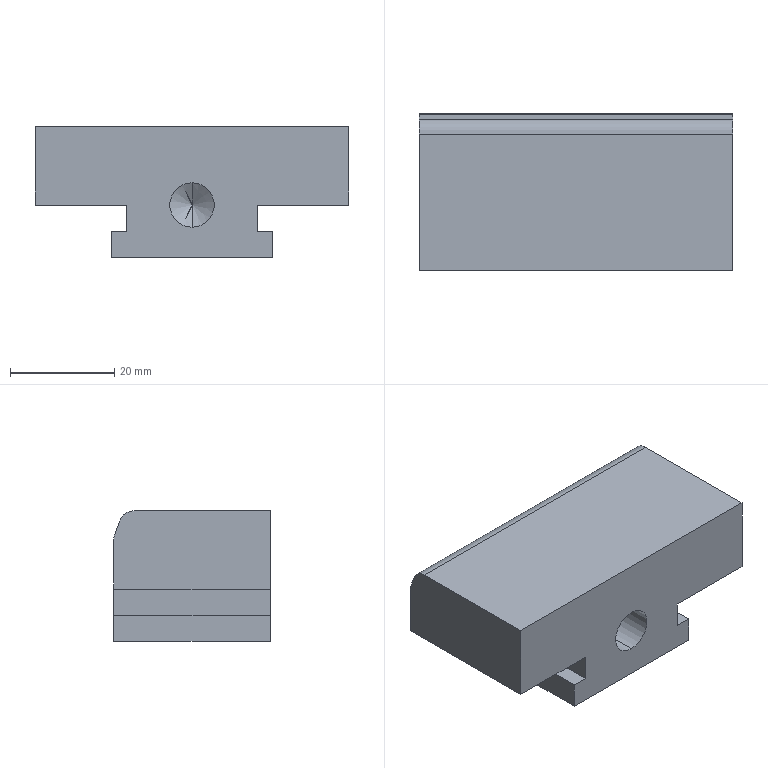Part | SolidWorks | features Chamfer 1, Cut 1, Extrusion 1, Fillet 1, HoleWzd 1, ICE 1 | 1 solid | 21 faces | box 60 x 30 x 25 mm | volume 33639 mm3 | plane 15 | cylinder 4 | cone 2 | commonest cylinder face diameters 6 x2 8.5 x2
STEP:
#1=CARTESIAN_POINT('',(-16.517,24.697,14.25));
#2=VERTEX_POINT('',#1);
#3=CARTESIAN_POINT('',(-16.517,24.697,5.75));
#4=VERTEX_POINT('',#3);
#5=CARTESIAN_POINT('',(-16.517,24.697,10.));
#6=DIRECTION('',(0.,-1.,0.));
#7=DIRECTION('',(0.,0.,-1.));
#8=AXIS2_PLACEMENT_3D('',#5,#6,#7);
#9=CIRCLE('',#8,4.25);
#10=EDGE_CURVE('',#2,#4,#9,.T.);
#11=ORIENTED_EDGE('',*,*,#10,.F.);
#12=CARTESIAN_POINT('',(-16.517,0.1974,14.25));
#13=VERTEX_POINT('',#12);
#14=CARTESIAN_POINT('',(-16.517,0.1974,14.25));
#15=DIRECTION('',(0.,-1.,0.));
#16=VECTOR('',#15,1000.);
#17=LINE('',#14,#16);
#18=EDGE_CURVE('',#2,#13,#17,.T.);
#19=ORIENTED_EDGE('',*,*,#18,.T.);
#20=CARTESIAN_POINT('',(-16.517,0.1974,5.75));
#21=VERTEX_POINT('',#20);
#22=CARTESIAN_POINT('',(-16.517,0.1974,10.));
#23=DIRECTION('',(0.,-1.,0.));
#24=DIRECTION('',(0.,0.,-1.));
#25=AXIS2_PLACEMENT_3D('',#22,#23,#24);
#26=CIRCLE('',#25,4.25);
#27=EDGE_CURVE('',#13,#21,#26,.T.);
#28=ORIENTED_EDGE('',*,*,#27,.T.);
#29=CARTESIAN_POINT('',(-16.517,0.1974,5.75));
#30=DIRECTION('',(0.,-1.,0.));
#31=VECTOR('',#30,1000.);
#32=LINE('',#29,#31);
#33=EDGE_CURVE('',#4,#21,#32,.T.);
#34=ORIENTED_EDGE('',*,*,#33,.F.);
#35=EDGE_LOOP('',(#11,#19,#28,#34));
#36=FACE_OUTER_BOUND('',#35,.T.);
#37=CARTESIAN_POINT('',(-16.517,0.1974,10.));
#38=DIRECTION('',(0.,-1.,0.));
#39=DIRECTION('',(0.,0.,-1.));
#40=AXIS2_PLACEMENT_3D('',#37,#38,#39);
#41=CYLINDRICAL_SURFACE('',#40,4.25);
#42=ADVANCED_FACE('',(#36),#41,.F.);
#43=CARTESIAN_POINT('',(-16.517,27.251,10.));
#44=VERTEX_POINT('',#43);
#45=CARTESIAN_POINT('',(-16.517,24.697,5.75));
#46=DIRECTION('',(0.,-0.515,-0.8572));
#47=VECTOR('',#46,1000.);
#48=LINE('',#45,#47);
#49=EDGE_CURVE('',#44,#4,#48,.T.);
#50=ORIENTED_EDGE('',*,*,#49,.F.);
#51=CARTESIAN_POINT('',(-16.517,24.697,14.25));
#52=DIRECTION('',(0.,-0.515,0.8572));
#53=VECTOR('',#52,1000.);
#54=LINE('',#51,#53);
#55=EDGE_CURVE('',#44,#2,#54,.T.);
#56=ORIENTED_EDGE('',*,*,#55,.T.);
#57=ORIENTED_EDGE('',*,*,#10,.T.);
#58=EDGE_LOOP('',(#50,#56,#57));
#59=FACE_OUTER_BOUND('',#58,.T.);
#60=CARTESIAN_POINT('',(-16.517,24.697,10.));
#61=DIRECTION('',(0.,-1.,0.));
#62=DIRECTION('',(0.,0.,-1.));
#63=AXIS2_PLACEMENT_3D('',#60,#61,#62);
#64=CONICAL_SURFACE('',#63,4.25,1.03);
#65=ADVANCED_FACE('',(#59),#64,.F.);
#66=CARTESIAN_POINT('',(-32.017,0.1974,5.));
#67=VERTEX_POINT('',#66);
#68=CARTESIAN_POINT('',(-32.017,0.1974,0.));
#69=VERTEX_POINT('',#68);
#70=CARTESIAN_POINT('',(-32.017,0.1974,25.));
#71=DIRECTION('',(0.,0.,-1.));
#72=VECTOR('',#71,1000.);
#73=LINE('',#70,#72);
#74=EDGE_CURVE('',#67,#69,#73,.T.);
#75=ORIENTED_EDGE('',*,*,#74,.F.);
#76=CARTESIAN_POINT('',(-32.017,30.197,5.));
#77=VERTEX_POINT('',#76);
#78=CARTESIAN_POINT('',(-32.017,30.197,5.));
#79=DIRECTION('',(0.,-1.,0.));
#80=VECTOR('',#79,1000.);
#81=LINE('',#78,#80);
#82=EDGE_CURVE('',#77,#67,#81,.T.);
#83=ORIENTED_EDGE('',*,*,#82,.F.);
#84=CARTESIAN_POINT('',(-32.017,30.197,0.));
#85=VERTEX_POINT('',#84);
#86=CARTESIAN_POINT('',(-32.017,30.197,25.));
#87=DIRECTION('',(0.,0.,-1.));
#88=VECTOR('',#87,1000.);
#89=LINE('',#86,#88);
#90=EDGE_CURVE('',#77,#85,#89,.T.);
#91=ORIENTED_EDGE('',*,*,#90,.T.);
#92=CARTESIAN_POINT('',(-32.017,30.197,0.));
#93=DIRECTION('',(0.,-1.,0.));
#94=VECTOR('',#93,1000.);
#95=LINE('',#92,#94);
#96=EDGE_CURVE('',#85,#69,#95,.T.);
#97=ORIENTED_EDGE('',*,*,#96,.T.);
#98=EDGE_LOOP('',(#75,#83,#91,#97));
#99=FACE_OUTER_BOUND('',#98,.T.);
#100=CARTESIAN_POINT('',(-32.017,30.197,25.));
#101=DIRECTION('',(1.,0.,0.));
#102=DIRECTION('',(0.,1.,0.));
#103=AXIS2_PLACEMENT_3D('',#100,#101,#102);
#104=PLANE('',#103);
#105=ADVANCED_FACE('',(#99),#104,.F.);
#106=CARTESIAN_POINT('',(-16.517,0.1974,10.));
#107=DIRECTION('',(0.,-1.,0.));
#108=DIRECTION('',(0.,0.,-1.));
#109=AXIS2_PLACEMENT_3D('',#106,#107,#108);
#110=CIRCLE('',#109,4.25);
#111=EDGE_CURVE('',#21,#13,#110,.T.);
#112=ORIENTED_EDGE('',*,*,#111,.F.);
#113=ORIENTED_EDGE('',*,*,#27,.F.);
#114=EDGE_LOOP('',(#112,#113));
#115=FACE_BOUND('',#114,.T.);
#116=CARTESIAN_POINT('',(-4.017,0.1974,5.));
#117=VERTEX_POINT('',#116);
#118=CARTESIAN_POINT('',(-1.017,0.1974,5.));
#119=VERTEX_POINT('',#118);
#120=CARTESIAN_POINT('',(-4.017,0.1974,5.));
#121=DIRECTION('',(1.,0.,0.));
#122=VECTOR('',#121,1000.);
#123=LINE('',#120,#122);
#124=EDGE_CURVE('',#117,#119,#123,.T.);
#125=ORIENTED_EDGE('',*,*,#124,.F.);
#126=CARTESIAN_POINT('',(-4.017,0.1974,10.));
#127=VERTEX_POINT('',#126);
#128=CARTESIAN_POINT('',(-4.017,0.1974,5.));
#129=DIRECTION('',(0.,0.,-1.));
#130=VECTOR('',#129,1000.);
#131=LINE('',#128,#130);
#132=EDGE_CURVE('',#127,#117,#131,.T.);
#133=ORIENTED_EDGE('',*,*,#132,.F.);
#134=CARTESIAN_POINT('',(13.483,0.1974,10.));
#135=VERTEX_POINT('',#134);
#136=CARTESIAN_POINT('',(-4.017,0.1974,10.));
#137=DIRECTION('',(-1.,0.,0.));
#138=VECTOR('',#137,1000.);
#139=LINE('',#136,#138);
#140=EDGE_CURVE('',#135,#127,#139,.T.);
#141=ORIENTED_EDGE('',*,*,#140,.F.);
#142=CARTESIAN_POINT('',(13.483,0.1974,25.));
#143=VERTEX_POINT('',#142);
#144=CARTESIAN_POINT('',(13.483,0.1974,25.));
#145=DIRECTION('',(0.,0.,-1.));
#146=VECTOR('',#145,1000.);
#147=LINE('',#144,#146);
#148=EDGE_CURVE('',#143,#135,#147,.T.);
#149=ORIENTED_EDGE('',*,*,#148,.F.);
#150=CARTESIAN_POINT('',(-46.517,0.1974,25.));
#151=VERTEX_POINT('',#150);
#152=CARTESIAN_POINT('',(-32.017,0.1974,25.));
#153=DIRECTION('',(1.,0.,0.));
#154=VECTOR('',#153,1000.);
#155=LINE('',#152,#154);
#156=EDGE_CURVE('',#151,#143,#155,.T.);
#157=ORIENTED_EDGE('',*,*,#156,.F.);
#158=CARTESIAN_POINT('',(-46.517,0.1974,10.));
#159=VERTEX_POINT('',#158);
#160=CARTESIAN_POINT('',(-46.517,0.1974,25.));
#161=DIRECTION('',(0.,0.,1.));
#162=VECTOR('',#161,1000.);
#163=LINE('',#160,#162);
#164=EDGE_CURVE('',#159,#151,#163,.T.);
#165=ORIENTED_EDGE('',*,*,#164,.F.);
#166=CARTESIAN_POINT('',(-29.017,0.1974,10.));
#167=VERTEX_POINT('',#166);
#168=CARTESIAN_POINT('',(-29.017,0.1974,10.));
#169=DIRECTION('',(-1.,0.,0.));
#170=VECTOR('',#169,1000.);
#171=LINE('',#168,#170);
#172=EDGE_CURVE('',#167,#159,#171,.T.);
#173=ORIENTED_EDGE('',*,*,#172,.F.);
#174=CARTESIAN_POINT('',(-29.017,0.1974,5.));
#175=VERTEX_POINT('',#174);
#176=CARTESIAN_POINT('',(-29.017,0.1974,5.));
#177=DIRECTION('',(0.,0.,1.));
#178=VECTOR('',#177,1000.);
#179=LINE('',#176,#178);
#180=EDGE_CURVE('',#175,#167,#179,.T.);
#181=ORIENTED_EDGE('',*,*,#180,.F.);
#182=CARTESIAN_POINT('',(-29.017,0.1974,5.));
#183=DIRECTION('',(1.,0.,0.));
#184=VECTOR('',#183,1000.);
#185=LINE('',#182,#184);
#186=EDGE_CURVE('',#67,#175,#185,.T.);
#187=ORIENTED_EDGE('',*,*,#186,.F.);
#188=ORIENTED_EDGE('',*,*,#74,.T.);
#189=CARTESIAN_POINT('',(-1.017,0.1974,0.));
#190=VERTEX_POINT('',#189);
#191=CARTESIAN_POINT('',(-32.017,0.1974,0.));
#192=DIRECTION('',(1.,0.,0.));
#193=VECTOR('',#192,1000.);
#194=LINE('',#191,#193);
#195=EDGE_CURVE('',#69,#190,#194,.T.);
#196=ORIENTED_EDGE('',*,*,#195,.T.);
#197=CARTESIAN_POINT('',(-1.017,0.1974,25.));
#198=DIRECTION('',(0.,0.,-1.));
#199=VECTOR('',#198,1000.);
#200=LINE('',#197,#199);
#201=EDGE_CURVE('',#119,#190,#200,.T.);
#202=ORIENTED_EDGE('',*,*,#201,.F.);
#203=EDGE_LOOP('',(#125,#133,#141,#149,#157,#165,#173,#181,#187,#188,#196,#202));
#204=FACE_OUTER_BOUND('',#203,.T.);
#205=CARTESIAN_POINT('',(-32.017,0.1974,25.));
#206=DIRECTION('',(0.,1.,0.));
#207=DIRECTION('',(0.,0.,1.));
#208=AXIS2_PLACEMENT_3D('',#205,#206,#207);
#209=PLANE('',#208);
#210=ADVANCED_FACE('',(#115,#204),#209,.F.);
#211=CARTESIAN_POINT('',(-1.017,30.197,5.));
#212=VERTEX_POINT('',#211);
#213=CARTESIAN_POINT('',(-1.017,30.197,0.));
#214=VERTEX_POINT('',#213);
#215=CARTESIAN_POINT('',(-1.017,30.197,25.));
#216=DIRECTION('',(0.,0.,-1.));
#217=VECTOR('',#216,1000.);
#218=LINE('',#215,#217);
#219=EDGE_CURVE('',#212,#214,#218,.T.);
#220=ORIENTED_EDGE('',*,*,#219,.F.);
#221=CARTESIAN_POINT('',(-1.017,30.197,5.));
#222=DIRECTION('',(0.,-1.,0.));
#223=VECTOR('',#222,1000.);
#224=LINE('',#221,#223);
#225=EDGE_CURVE('',#212,#119,#224,.T.);
#226=ORIENTED_EDGE('',*,*,#225,.T.);
#227=ORIENTED_EDGE('',*,*,#201,.T.);
#228=CARTESIAN_POINT('',(-1.017,30.197,0.));
#229=DIRECTION('',(0.,1.,0.));
#230=VECTOR('',#229,1000.);
#231=LINE('',#228,#230);
#232=EDGE_CURVE('',#190,#214,#231,.T.);
#233=ORIENTED_EDGE('',*,*,#232,.T.);
#234=EDGE_LOOP('',(#220,#226,#227,#233));
#235=FACE_OUTER_BOUND('',#234,.T.);
#236=CARTESIAN_POINT('',(-1.017,30.197,25.));
#237=DIRECTION('',(-1.,0.,0.));
#238=DIRECTION('',(0.,-1.,0.));
#239=AXIS2_PLACEMENT_3D('',#236,#237,#238);
#240=PLANE('',#239);
#241=ADVANCED_FACE('',(#235),#240,.F.);
#242=CARTESIAN_POINT('',(-46.517,30.197,10.));
#243=VERTEX_POINT('',#242);
#244=CARTESIAN_POINT('',(-46.517,30.197,19.471));
#245=VERTEX_POINT('',#244);
#246=CARTESIAN_POINT('',(-46.517,30.197,25.));
#247=DIRECTION('',(0.,0.,1.));
#248=VECTOR('',#247,1000.);
#249=LINE('',#246,#248);
#250=EDGE_CURVE('',#243,#245,#249,.T.);
#251=ORIENTED_EDGE('',*,*,#250,.T.);
#252=CARTESIAN_POINT('',(13.483,30.197,19.471));
#253=VERTEX_POINT('',#252);
#254=CARTESIAN_POINT('',(13.483,30.197,19.471));
#255=DIRECTION('',(1.,0.,0.));
#256=VECTOR('',#255,1000.);
#257=LINE('',#254,#256);
#258=EDGE_CURVE('',#245,#253,#257,.T.);
#259=ORIENTED_EDGE('',*,*,#258,.T.);
#260=CARTESIAN_POINT('',(13.483,30.197,10.));
#261=VERTEX_POINT('',#260);
#262=CARTESIAN_POINT('',(13.483,30.197,25.));
#263=DIRECTION('',(0.,0.,-1.));
#264=VECTOR('',#263,1000.);
#265=LINE('',#262,#264);
#266=EDGE_CURVE('',#253,#261,#265,.T.);
#267=ORIENTED_EDGE('',*,*,#266,.T.);
#268=CARTESIAN_POINT('',(-4.017,30.197,10.));
#269=VERTEX_POINT('',#268);
#270=CARTESIAN_POINT('',(-4.017,30.197,10.));
#271=DIRECTION('',(-1.,0.,0.));
#272=VECTOR('',#271,1000.);
#273=LINE('',#270,#272);
#274=EDGE_CURVE('',#261,#269,#273,.T.);
#275=ORIENTED_EDGE('',*,*,#274,.T.);
#276=CARTESIAN_POINT('',(-4.017,30.197,5.));
#277=VERTEX_POINT('',#276);
#278=CARTESIAN_POINT('',(-4.017,30.197,5.));
#279=DIRECTION('',(0.,0.,-1.));
#280=VECTOR('',#279,1000.);
#281=LINE('',#278,#280);
#282=EDGE_CURVE('',#269,#277,#281,.T.);
#283=ORIENTED_EDGE('',*,*,#282,.T.);
#284=CARTESIAN_POINT('',(-4.017,30.197,5.));
#285=DIRECTION('',(1.,0.,0.));
#286=VECTOR('',#285,1000.);
#287=LINE('',#284,#286);
#288=EDGE_CURVE('',#277,#212,#287,.T.);
#289=ORIENTED_EDGE('',*,*,#288,.T.);
#290=ORIENTED_EDGE('',*,*,#219,.T.);
#291=CARTESIAN_POINT('',(-32.017,30.197,0.));
#292=DIRECTION('',(-1.,0.,0.));
#293=VECTOR('',#292,1000.);
#294=LINE('',#291,#293);
#295=EDGE_CURVE('',#214,#85,#294,.T.);
#296=ORIENTED_EDGE('',*,*,#295,.T.);
#297=ORIENTED_EDGE('',*,*,#90,.F.);
#298=CARTESIAN_POINT('',(-29.017,30.197,5.));
#299=VERTEX_POINT('',#298);
#300=CARTESIAN_POINT('',(-29.017,30.197,5.));
#301=DIRECTION('',(1.,0.,0.));
#302=VECTOR('',#301,1000.);
#303=LINE('',#300,#302);
#304=EDGE_CURVE('',#77,#299,#303,.T.);
#305=ORIENTED_EDGE('',*,*,#304,.T.);
#306=CARTESIAN_POINT('',(-29.017,30.197,10.));
#307=VERTEX_POINT('',#306);
#308=CARTESIAN_POINT('',(-29.017,30.197,5.));
#309=DIRECTION('',(0.,0.,1.));
#310=VECTOR('',#309,1000.);
#311=LINE('',#308,#310);
#312=EDGE_CURVE('',#299,#307,#311,.T.);
#313=ORIENTED_EDGE('',*,*,#312,.T.);
#314=CARTESIAN_POINT('',(-29.017,30.197,10.));
#315=DIRECTION('',(-1.,0.,0.));
#316=VECTOR('',#315,1000.);
#317=LINE('',#314,#316);
#318=EDGE_CURVE('',#307,#243,#317,.T.);
#319=ORIENTED_EDGE('',*,*,#318,.T.);
#320=EDGE_LOOP('',(#251,#259,#267,#275,#283,#289,#290,#296,#297,#305,#313,#319));
#321=FACE_OUTER_BOUND('',#320,.T.);
#322=CARTESIAN_POINT('',(-32.017,30.197,25.));
#323=DIRECTION('',(0.,-1.,0.));
#324=DIRECTION('',(0.,0.,-1.));
#325=AXIS2_PLACEMENT_3D('',#322,#323,#324);
#326=PLANE('',#325);
#327=ADVANCED_FACE('',(#321),#326,.F.);
#328=CARTESIAN_POINT('',(13.483,26.277,25.));
#329=VERTEX_POINT('',#328);
#330=CARTESIAN_POINT('',(13.483,0.1974,25.));
#331=DIRECTION('',(0.,1.,0.));
#332=VECTOR('',#331,1000.);
#333=LINE('',#330,#332);
#334=EDGE_CURVE('',#143,#329,#333,.T.);
#335=ORIENTED_EDGE('',*,*,#334,.T.);
#336=CARTESIAN_POINT('',(-46.517,26.277,25.));
#337=VERTEX_POINT('',#336);
#338=CARTESIAN_POINT('',(0.,26.277,25.));
#339=DIRECTION('',(-1.,0.,0.));
#340=VECTOR('',#339,1000.);
#341=LINE('',#338,#340);
#342=EDGE_CURVE('',#329,#337,#341,.T.);
#343=ORIENTED_EDGE('',*,*,#342,.T.);
#344=CARTESIAN_POINT('',(-46.517,0.1974,25.));
#345=DIRECTION('',(0.,1.,0.));
#346=VECTOR('',#345,1000.);
#347=LINE('',#344,#346);
#348=EDGE_CURVE('',#151,#337,#347,.T.);
#349=ORIENTED_EDGE('',*,*,#348,.F.);
#350=ORIENTED_EDGE('',*,*,#156,.T.);
#351=EDGE_LOOP('',(#335,#343,#349,#350));
#352=FACE_OUTER_BOUND('',#351,.T.);
#353=CARTESIAN_POINT('',(0.,0.,25.));
#354=DIRECTION('',(0.,0.,1.));
#355=DIRECTION('',(1.,0.,0.));
#356=AXIS2_PLACEMENT_3D('',#353,#354,#355);
#357=PLANE('',#356);
#358=ADVANCED_FACE('',(#352),#357,.T.);
#359=ORIENTED_EDGE('',*,*,#96,.F.);
#360=ORIENTED_EDGE('',*,*,#295,.F.);
#361=ORIENTED_EDGE('',*,*,#232,.F.);
#362=ORIENTED_EDGE('',*,*,#195,.F.);
#363=EDGE_LOOP('',(#359,#360,#361,#362));
#364=FACE_OUTER_BOUND('',#363,.T.);
#365=CARTESIAN_POINT('',(0.,0.,0.));
#366=DIRECTION('',(0.,0.,1.));
#367=DIRECTION('',(1.,0.,0.));
#368=AXIS2_PLACEMENT_3D('',#365,#366,#367);
#369=PLANE('',#368);
#370=ADVANCED_FACE('',(#364),#369,.F.);
#371=ORIENTED_EDGE('',*,*,#180,.T.);
#372=CARTESIAN_POINT('',(-29.017,0.1974,10.));
#373=DIRECTION('',(0.,1.,0.));
#374=VECTOR('',#373,1000.);
#375=LINE('',#372,#374);
#376=EDGE_CURVE('',#167,#307,#375,.T.);
#377=ORIENTED_EDGE('',*,*,#376,.T.);
#378=ORIENTED_EDGE('',*,*,#312,.F.);
#379=CARTESIAN_POINT('',(-29.017,30.197,5.));
#380=DIRECTION('',(0.,-1.,0.));
#381=VECTOR('',#380,1000.);
#382=LINE('',#379,#381);
#383=EDGE_CURVE('',#299,#175,#382,.T.);
#384=ORIENTED_EDGE('',*,*,#383,.T.);
#385=EDGE_LOOP('',(#371,#377,#378,#384));
#386=FACE_OUTER_BOUND('',#385,.T.);
#387=CARTESIAN_POINT('',(-29.017,30.197,5.));
#388=DIRECTION('',(1.,0.,0.));
#389=DIRECTION('',(0.,1.,0.));
#390=AXIS2_PLACEMENT_3D('',#387,#388,#389);
#391=PLANE('',#390);
#392=ADVANCED_FACE('',(#386),#391,.F.);
#393=ORIENTED_EDGE('',*,*,#186,.T.);
#394=ORIENTED_EDGE('',*,*,#383,.F.);
#395=ORIENTED_EDGE('',*,*,#304,.F.);
#396=ORIENTED_EDGE('',*,*,#82,.T.);
#397=EDGE_LOOP('',(#393,#394,#395,#396));
#398=FACE_OUTER_BOUND('',#397,.T.);
#399=CARTESIAN_POINT('',(-29.017,30.197,5.));
#400=DIRECTION('',(0.,0.,-1.));
#401=DIRECTION('',(-1.,0.,0.));
#402=AXIS2_PLACEMENT_3D('',#399,#400,#401);
#403=PLANE('',#402);
#404=ADVANCED_FACE('',(#398),#403,.F.);
#405=ORIENTED_EDGE('',*,*,#282,.F.);
#406=CARTESIAN_POINT('',(-4.017,0.1974,10.));
#407=DIRECTION('',(0.,1.,0.));
#408=VECTOR('',#407,1000.);
#409=LINE('',#406,#408);
#410=EDGE_CURVE('',#127,#269,#409,.T.);
#411=ORIENTED_EDGE('',*,*,#410,.F.);
#412=ORIENTED_EDGE('',*,*,#132,.T.);
#413=CARTESIAN_POINT('',(-4.017,30.197,5.));
#414=DIRECTION('',(0.,-1.,0.));
#415=VECTOR('',#414,1000.);
#416=LINE('',#413,#415);
#417=EDGE_CURVE('',#277,#117,#416,.T.);
#418=ORIENTED_EDGE('',*,*,#417,.F.);
#419=EDGE_LOOP('',(#405,#411,#412,#418));
#420=FACE_OUTER_BOUND('',#419,.T.);
#421=CARTESIAN_POINT('',(-4.017,30.197,5.));
#422=DIRECTION('',(-1.,0.,0.));
#423=DIRECTION('',(0.,-1.,0.));
#424=AXIS2_PLACEMENT_3D('',#421,#422,#423);
#425=PLANE('',#424);
#426=ADVANCED_FACE('',(#420),#425,.F.);
#427=ORIENTED_EDGE('',*,*,#124,.T.);
#428=ORIENTED_EDGE('',*,*,#225,.F.);
#429=ORIENTED_EDGE('',*,*,#288,.F.);
#430=ORIENTED_EDGE('',*,*,#417,.T.);
#431=EDGE_LOOP('',(#427,#428,#429,#430));
#432=FACE_OUTER_BOUND('',#431,.T.);
#433=CARTESIAN_POINT('',(-4.017,30.197,5.));
#434=DIRECTION('',(0.,0.,-1.));
#435=DIRECTION('',(-1.,0.,0.));
#436=AXIS2_PLACEMENT_3D('',#433,#434,#435);
#437=PLANE('',#436);
#438=ADVANCED_FACE('',(#432),#437,.F.);
#439=ORIENTED_EDGE('',*,*,#274,.F.);
#440=CARTESIAN_POINT('',(13.483,0.1974,10.));
#441=DIRECTION('',(0.,1.,0.));
#442=VECTOR('',#441,1000.);
#443=LINE('',#440,#442);
#444=EDGE_CURVE('',#135,#261,#443,.T.);
#445=ORIENTED_EDGE('',*,*,#444,.F.);
#446=ORIENTED_EDGE('',*,*,#140,.T.);
#447=ORIENTED_EDGE('',*,*,#410,.T.);
#448=EDGE_LOOP('',(#439,#445,#446,#447));
#449=FACE_OUTER_BOUND('',#448,.T.);
#450=CARTESIAN_POINT('',(-4.017,0.1974,10.));
#451=DIRECTION('',(0.,0.,-1.));
#452=DIRECTION('',(-1.,0.,0.));
#453=AXIS2_PLACEMENT_3D('',#450,#451,#452);
#454=PLANE('',#453);
#455=ADVANCED_FACE('',(#449),#454,.T.);
#456=CARTESIAN_POINT('',(13.483,30.016,20.497));
#457=VERTEX_POINT('',#456);
#458=CARTESIAN_POINT('',(13.483,29.096,23.026));
#459=VERTEX_POINT('',#458);
#460=CARTESIAN_POINT('',(13.483,25.081,34.057));
#461=DIRECTION('',(0.,-0.342,0.9397));
#462=VECTOR('',#461,1000.);
#463=LINE('',#460,#462);
#464=EDGE_CURVE('',#457,#459,#463,.T.);
#465=ORIENTED_EDGE('',*,*,#464,.T.);
#466=CARTESIAN_POINT('',(13.483,26.277,22.));
#467=DIRECTION('',(1.,0.,0.));
#468=DIRECTION('',(0.,0.,-1.));
#469=AXIS2_PLACEMENT_3D('',#466,#467,#468);
#470=CIRCLE('',#469,3.);
#471=EDGE_CURVE('',#459,#329,#470,.T.);
#472=ORIENTED_EDGE('',*,*,#471,.T.);
#473=ORIENTED_EDGE('',*,*,#334,.F.);
#474=ORIENTED_EDGE('',*,*,#148,.T.);
#475=ORIENTED_EDGE('',*,*,#444,.T.);
#476=ORIENTED_EDGE('',*,*,#266,.F.);
#477=CARTESIAN_POINT('',(13.483,27.197,19.471));
#478=DIRECTION('',(1.,0.,0.));
#479=DIRECTION('',(0.,0.,-1.));
#480=AXIS2_PLACEMENT_3D('',#477,#478,#479);
#481=CIRCLE('',#480,3.);
#482=EDGE_CURVE('',#253,#457,#481,.T.);
#483=ORIENTED_EDGE('',*,*,#482,.T.);
#484=EDGE_LOOP('',(#465,#472,#473,#474,#475,#476,#483));
#485=FACE_OUTER_BOUND('',#484,.T.);
#486=CARTESIAN_POINT('',(13.483,0.1974,25.));
#487=DIRECTION('',(1.,0.,0.));
#488=DIRECTION('',(0.,0.,-1.));
#489=AXIS2_PLACEMENT_3D('',#486,#487,#488);
#490=PLANE('',#489);
#491=ADVANCED_FACE('',(#485),#490,.T.);
#492=ORIENTED_EDGE('',*,*,#348,.T.);
#493=CARTESIAN_POINT('',(-46.517,29.096,23.026));
#494=VERTEX_POINT('',#493);
#495=CARTESIAN_POINT('',(-46.517,26.277,22.));
#496=DIRECTION('',(-1.,0.,0.));
#497=DIRECTION('',(0.,0.,1.));
#498=AXIS2_PLACEMENT_3D('',#495,#496,#497);
#499=CIRCLE('',#498,3.);
#500=EDGE_CURVE('',#337,#494,#499,.T.);
#501=ORIENTED_EDGE('',*,*,#500,.T.);
#502=CARTESIAN_POINT('',(-46.517,30.016,20.497));
#503=VERTEX_POINT('',#502);
#504=CARTESIAN_POINT('',(-46.517,25.081,34.057));
#505=DIRECTION('',(0.,0.342,-0.9397));
#506=VECTOR('',#505,1000.);
#507=LINE('',#504,#506);
#508=EDGE_CURVE('',#494,#503,#507,.T.);
#509=ORIENTED_EDGE('',*,*,#508,.T.);
#510=CARTESIAN_POINT('',(-46.517,27.197,19.471));
#511=DIRECTION('',(-1.,0.,0.));
#512=DIRECTION('',(0.,0.,1.));
#513=AXIS2_PLACEMENT_3D('',#510,#511,#512);
#514=CIRCLE('',#513,3.);
#515=EDGE_CURVE('',#503,#245,#514,.T.);
#516=ORIENTED_EDGE('',*,*,#515,.T.);
#517=ORIENTED_EDGE('',*,*,#250,.F.);
#518=CARTESIAN_POINT('',(-46.517,0.1974,10.));
#519=DIRECTION('',(0.,1.,0.));
#520=VECTOR('',#519,1000.);
#521=LINE('',#518,#520);
#522=EDGE_CURVE('',#159,#243,#521,.T.);
#523=ORIENTED_EDGE('',*,*,#522,.F.);
#524=ORIENTED_EDGE('',*,*,#164,.T.);
#525=EDGE_LOOP('',(#492,#501,#509,#516,#517,#523,#524));
#526=FACE_OUTER_BOUND('',#525,.T.);
#527=CARTESIAN_POINT('',(-46.517,0.1974,25.));
#528=DIRECTION('',(-1.,0.,0.));
#529=DIRECTION('',(0.,0.,1.));
#530=AXIS2_PLACEMENT_3D('',#527,#528,#529);
#531=PLANE('',#530);
#532=ADVANCED_FACE('',(#526),#531,.T.);
#533=ORIENTED_EDGE('',*,*,#318,.F.);
#534=ORIENTED_EDGE('',*,*,#376,.F.);
#535=ORIENTED_EDGE('',*,*,#172,.T.);
#536=ORIENTED_EDGE('',*,*,#522,.T.);
#537=EDGE_LOOP('',(#533,#534,#535,#536));
#538=FACE_OUTER_BOUND('',#537,.T.);
#539=CARTESIAN_POINT('',(-29.017,0.1974,10.));
#540=DIRECTION('',(0.,0.,-1.));
#541=DIRECTION('',(-1.,0.,0.));
#542=AXIS2_PLACEMENT_3D('',#539,#540,#541);
#543=PLANE('',#542);
#544=ADVANCED_FACE('',(#538),#543,.T.);
#545=ORIENTED_EDGE('',*,*,#508,.F.);
#546=CARTESIAN_POINT('',(0.,29.096,23.026));
#547=DIRECTION('',(1.,0.,0.));
#548=VECTOR('',#547,1000.);
#549=LINE('',#546,#548);
#550=EDGE_CURVE('',#494,#459,#549,.T.);
#551=ORIENTED_EDGE('',*,*,#550,.T.);
#552=ORIENTED_EDGE('',*,*,#464,.F.);
#553=CARTESIAN_POINT('',(-46.517,30.016,20.497));
#554=DIRECTION('',(-1.,0.,0.));
#555=VECTOR('',#554,1000.);
#556=LINE('',#553,#555);
#557=EDGE_CURVE('',#457,#503,#556,.T.);
#558=ORIENTED_EDGE('',*,*,#557,.T.);
#559=EDGE_LOOP('',(#545,#551,#552,#558));
#560=FACE_OUTER_BOUND('',#559,.T.);
#561=CARTESIAN_POINT('',(0.,28.378,25.));
#562=DIRECTION('',(0.,0.9397,0.342));
#563=DIRECTION('',(1.,0.,0.));
#564=AXIS2_PLACEMENT_3D('',#561,#562,#563);
#565=PLANE('',#564);
#566=ADVANCED_FACE('',(#560),#565,.T.);
#567=ORIENTED_EDGE('',*,*,#471,.F.);
#568=ORIENTED_EDGE('',*,*,#550,.F.);
#569=ORIENTED_EDGE('',*,*,#500,.F.);
#570=ORIENTED_EDGE('',*,*,#342,.F.);
#571=EDGE_LOOP('',(#567,#568,#569,#570));
#572=FACE_OUTER_BOUND('',#571,.T.);
#573=CARTESIAN_POINT('',(0.,26.277,22.));
#574=DIRECTION('',(-1.,0.,0.));
#575=DIRECTION('',(0.,0.,1.));
#576=AXIS2_PLACEMENT_3D('',#573,#574,#575);
#577=CYLINDRICAL_SURFACE('',#576,3.);
#578=ADVANCED_FACE('',(#572),#577,.T.);
#579=ORIENTED_EDGE('',*,*,#515,.F.);
#580=ORIENTED_EDGE('',*,*,#557,.F.);
#581=ORIENTED_EDGE('',*,*,#482,.F.);
#582=ORIENTED_EDGE('',*,*,#258,.F.);
#583=EDGE_LOOP('',(#579,#580,#581,#582));
#584=FACE_OUTER_BOUND('',#583,.T.);
#585=CARTESIAN_POINT('',(-32.017,27.197,19.471));
#586=DIRECTION('',(-1.,0.,0.));
#587=DIRECTION('',(0.,0.,1.));
#588=AXIS2_PLACEMENT_3D('',#585,#586,#587);
#589=CYLINDRICAL_SURFACE('',#588,3.);
#590=ADVANCED_FACE('',(#584),#589,.T.);
#591=ORIENTED_EDGE('',*,*,#55,.F.);
#592=ORIENTED_EDGE('',*,*,#49,.T.);
#593=CARTESIAN_POINT('',(-16.517,24.697,10.));
#594=DIRECTION('',(0.,-1.,0.));
#595=DIRECTION('',(0.,0.,-1.));
#596=AXIS2_PLACEMENT_3D('',#593,#594,#595);
#597=CIRCLE('',#596,4.25);
#598=EDGE_CURVE('',#4,#2,#597,.T.);
#599=ORIENTED_EDGE('',*,*,#598,.T.);
#600=EDGE_LOOP('',(#591,#592,#599));
#601=FACE_OUTER_BOUND('',#600,.T.);
#602=CARTESIAN_POINT('',(-16.517,24.697,10.));
#603=DIRECTION('',(0.,-1.,0.));
#604=DIRECTION('',(0.,0.,-1.));
#605=AXIS2_PLACEMENT_3D('',#602,#603,#604);
#606=CONICAL_SURFACE('',#605,4.25,1.03);
#607=ADVANCED_FACE('',(#601),#606,.F.);
#608=ORIENTED_EDGE('',*,*,#18,.F.);
#609=ORIENTED_EDGE('',*,*,#598,.F.);
#610=ORIENTED_EDGE('',*,*,#33,.T.);
#611=ORIENTED_EDGE('',*,*,#111,.T.);
#612=EDGE_LOOP('',(#608,#609,#610,#611));
#613=FACE_OUTER_BOUND('',#612,.T.);
#614=CARTESIAN_POINT('',(-16.517,0.1974,10.));
#615=DIRECTION('',(0.,-1.,0.));
#616=DIRECTION('',(0.,0.,-1.));
#617=AXIS2_PLACEMENT_3D('',#614,#615,#616);
#618=CYLINDRICAL_SURFACE('',#617,4.25);
#619=ADVANCED_FACE('',(#613),#618,.F.);
#620=CLOSED_SHELL('',(#42,#65,#105,#210,#241,#327,#358,#370,#392,#404,#426,#438,#455,#491,#532,#544,#566,#578,#590,#607,#619));
#621=MANIFOLD_SOLID_BREP('',#620);
#622=CARTESIAN_POINT('',(0.,0.,0.));
#623=DIRECTION('',(0.,0.,1.));
#624=DIRECTION('',(1.,0.,0.));
#625=AXIS2_PLACEMENT_3D('',#622,#623,#624);
#626=(LENGTH_UNIT()NAMED_UNIT(*)SI_UNIT(.MILLI.,.METRE.));
#627=UNCERTAINTY_MEASURE_WITH_UNIT(LENGTH_MEASURE(0.00001),#626,'','');
#628=(NAMED_UNIT(*)PLANE_ANGLE_UNIT()SI_UNIT($,.RADIAN.));
#629=(NAMED_UNIT(*)SI_UNIT($,.STERADIAN.)SOLID_ANGLE_UNIT());
#630=(GEOMETRIC_REPRESENTATION_CONTEXT(3)GLOBAL_UNCERTAINTY_ASSIGNED_CONTEXT((#627))GLOBAL_UNIT_ASSIGNED_CONTEXT((#626,#628,#629))REPRESENTATION_CONTEXT('',''));
#631=ADVANCED_BREP_SHAPE_REPRESENTATION('',(#621,#625),#630);